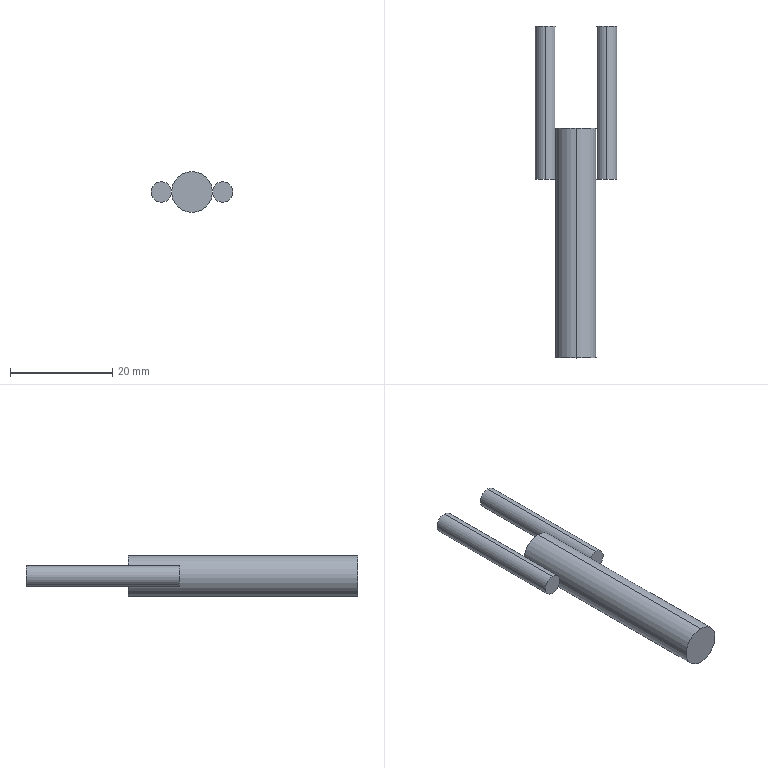Part | 3 solids | 12 faces | box 16 x 65 x 8 mm | volume 3016 mm3 | cylinder 6 | plane 6 | commonest cylinder face diameters 4 x4 8 x2
STEP:
#1=CARTESIAN_POINT('',(0.,45.,4.));
#2=VERTEX_POINT('',#1);
#3=CARTESIAN_POINT('',(0.,45.,-4.));
#4=VERTEX_POINT('',#3);
#5=CARTESIAN_POINT('',(0.,45.,0.));
#6=DIRECTION('',(0.,1.,0.));
#7=DIRECTION('',(0.,0.,1.));
#8=AXIS2_PLACEMENT_3D('',#5,#6,#7);
#9=CIRCLE('',#8,4.);
#10=EDGE_CURVE('',#2,#4,#9,.T.);
#11=ORIENTED_EDGE('',*,*,#10,.F.);
#12=CARTESIAN_POINT('',(0.,0.,4.));
#13=VERTEX_POINT('',#12);
#14=CARTESIAN_POINT('',(0.,45.,4.));
#15=DIRECTION('',(0.,-1.,0.));
#16=VECTOR('',#15,1000.);
#17=LINE('',#14,#16);
#18=EDGE_CURVE('',#2,#13,#17,.T.);
#19=ORIENTED_EDGE('',*,*,#18,.T.);
#20=CARTESIAN_POINT('',(0.,0.,-4.));
#21=VERTEX_POINT('',#20);
#22=CARTESIAN_POINT('',(0.,0.,0.));
#23=DIRECTION('',(0.,1.,0.));
#24=DIRECTION('',(0.,0.,1.));
#25=AXIS2_PLACEMENT_3D('',#22,#23,#24);
#26=CIRCLE('',#25,4.);
#27=EDGE_CURVE('',#13,#21,#26,.T.);
#28=ORIENTED_EDGE('',*,*,#27,.T.);
#29=CARTESIAN_POINT('',(0.,45.,-4.));
#30=DIRECTION('',(0.,-1.,0.));
#31=VECTOR('',#30,1000.);
#32=LINE('',#29,#31);
#33=EDGE_CURVE('',#4,#21,#32,.T.);
#34=ORIENTED_EDGE('',*,*,#33,.F.);
#35=EDGE_LOOP('',(#11,#19,#28,#34));
#36=FACE_OUTER_BOUND('',#35,.T.);
#37=CARTESIAN_POINT('',(0.,45.,0.));
#38=DIRECTION('',(0.,-1.,0.));
#39=DIRECTION('',(0.,0.,-1.));
#40=AXIS2_PLACEMENT_3D('',#37,#38,#39);
#41=CYLINDRICAL_SURFACE('',#40,4.);
#42=ADVANCED_FACE('',(#36),#41,.T.);
#43=ORIENTED_EDGE('',*,*,#18,.F.);
#44=CARTESIAN_POINT('',(0.,45.,0.));
#45=DIRECTION('',(0.,1.,0.));
#46=DIRECTION('',(0.,0.,1.));
#47=AXIS2_PLACEMENT_3D('',#44,#45,#46);
#48=CIRCLE('',#47,4.);
#49=EDGE_CURVE('',#4,#2,#48,.T.);
#50=ORIENTED_EDGE('',*,*,#49,.F.);
#51=ORIENTED_EDGE('',*,*,#33,.T.);
#52=CARTESIAN_POINT('',(0.,0.,0.));
#53=DIRECTION('',(0.,1.,0.));
#54=DIRECTION('',(0.,0.,1.));
#55=AXIS2_PLACEMENT_3D('',#52,#53,#54);
#56=CIRCLE('',#55,4.);
#57=EDGE_CURVE('',#21,#13,#56,.T.);
#58=ORIENTED_EDGE('',*,*,#57,.T.);
#59=EDGE_LOOP('',(#43,#50,#51,#58));
#60=FACE_OUTER_BOUND('',#59,.T.);
#61=CARTESIAN_POINT('',(0.,45.,0.));
#62=DIRECTION('',(0.,-1.,0.));
#63=DIRECTION('',(0.,0.,-1.));
#64=AXIS2_PLACEMENT_3D('',#61,#62,#63);
#65=CYLINDRICAL_SURFACE('',#64,4.);
#66=ADVANCED_FACE('',(#60),#65,.T.);
#67=ORIENTED_EDGE('',*,*,#49,.T.);
#68=ORIENTED_EDGE('',*,*,#10,.T.);
#69=EDGE_LOOP('',(#67,#68));
#70=FACE_OUTER_BOUND('',#69,.T.);
#71=CARTESIAN_POINT('',(0.,45.,0.));
#72=DIRECTION('',(0.,1.,0.));
#73=DIRECTION('',(0.,0.,1.));
#74=AXIS2_PLACEMENT_3D('',#71,#72,#73);
#75=PLANE('',#74);
#76=ADVANCED_FACE('',(#70),#75,.T.);
#77=ORIENTED_EDGE('',*,*,#57,.F.);
#78=ORIENTED_EDGE('',*,*,#27,.F.);
#79=EDGE_LOOP('',(#77,#78));
#80=FACE_OUTER_BOUND('',#79,.T.);
#81=CARTESIAN_POINT('',(0.,0.,0.));
#82=DIRECTION('',(0.,1.,0.));
#83=DIRECTION('',(0.,0.,1.));
#84=AXIS2_PLACEMENT_3D('',#81,#82,#83);
#85=PLANE('',#84);
#86=ADVANCED_FACE('',(#80),#85,.F.);
#87=CLOSED_SHELL('',(#42,#66,#76,#86));
#88=MANIFOLD_SOLID_BREP('',#87);
#89=CARTESIAN_POINT('',(-6.,65.,2.));
#90=VERTEX_POINT('',#89);
#91=CARTESIAN_POINT('',(-6.,65.,-2.));
#92=VERTEX_POINT('',#91);
#93=CARTESIAN_POINT('',(-6.,65.,0.));
#94=DIRECTION('',(0.,1.,0.));
#95=DIRECTION('',(0.,0.,1.));
#96=AXIS2_PLACEMENT_3D('',#93,#94,#95);
#97=CIRCLE('',#96,2.);
#98=EDGE_CURVE('',#90,#92,#97,.T.);
#99=ORIENTED_EDGE('',*,*,#98,.F.);
#100=CARTESIAN_POINT('',(-6.,35.,2.));
#101=VERTEX_POINT('',#100);
#102=CARTESIAN_POINT('',(-6.,65.,2.));
#103=DIRECTION('',(0.,-1.,0.));
#104=VECTOR('',#103,1000.);
#105=LINE('',#102,#104);
#106=EDGE_CURVE('',#90,#101,#105,.T.);
#107=ORIENTED_EDGE('',*,*,#106,.T.);
#108=CARTESIAN_POINT('',(-6.,35.,-2.));
#109=VERTEX_POINT('',#108);
#110=CARTESIAN_POINT('',(-6.,35.,0.));
#111=DIRECTION('',(0.,1.,0.));
#112=DIRECTION('',(0.,0.,1.));
#113=AXIS2_PLACEMENT_3D('',#110,#111,#112);
#114=CIRCLE('',#113,2.);
#115=EDGE_CURVE('',#101,#109,#114,.T.);
#116=ORIENTED_EDGE('',*,*,#115,.T.);
#117=CARTESIAN_POINT('',(-6.,65.,-2.));
#118=DIRECTION('',(0.,-1.,0.));
#119=VECTOR('',#118,1000.);
#120=LINE('',#117,#119);
#121=EDGE_CURVE('',#92,#109,#120,.T.);
#122=ORIENTED_EDGE('',*,*,#121,.F.);
#123=EDGE_LOOP('',(#99,#107,#116,#122));
#124=FACE_OUTER_BOUND('',#123,.T.);
#125=CARTESIAN_POINT('',(-6.,65.,0.));
#126=DIRECTION('',(0.,-1.,0.));
#127=DIRECTION('',(0.,0.,-1.));
#128=AXIS2_PLACEMENT_3D('',#125,#126,#127);
#129=CYLINDRICAL_SURFACE('',#128,2.);
#130=ADVANCED_FACE('',(#124),#129,.T.);
#131=ORIENTED_EDGE('',*,*,#106,.F.);
#132=CARTESIAN_POINT('',(-6.,65.,0.));
#133=DIRECTION('',(0.,1.,0.));
#134=DIRECTION('',(0.,0.,1.));
#135=AXIS2_PLACEMENT_3D('',#132,#133,#134);
#136=CIRCLE('',#135,2.);
#137=EDGE_CURVE('',#92,#90,#136,.T.);
#138=ORIENTED_EDGE('',*,*,#137,.F.);
#139=ORIENTED_EDGE('',*,*,#121,.T.);
#140=CARTESIAN_POINT('',(-6.,35.,0.));
#141=DIRECTION('',(0.,1.,0.));
#142=DIRECTION('',(0.,0.,1.));
#143=AXIS2_PLACEMENT_3D('',#140,#141,#142);
#144=CIRCLE('',#143,2.);
#145=EDGE_CURVE('',#109,#101,#144,.T.);
#146=ORIENTED_EDGE('',*,*,#145,.T.);
#147=EDGE_LOOP('',(#131,#138,#139,#146));
#148=FACE_OUTER_BOUND('',#147,.T.);
#149=CARTESIAN_POINT('',(-6.,65.,0.));
#150=DIRECTION('',(0.,-1.,0.));
#151=DIRECTION('',(0.,0.,-1.));
#152=AXIS2_PLACEMENT_3D('',#149,#150,#151);
#153=CYLINDRICAL_SURFACE('',#152,2.);
#154=ADVANCED_FACE('',(#148),#153,.T.);
#155=ORIENTED_EDGE('',*,*,#137,.T.);
#156=ORIENTED_EDGE('',*,*,#98,.T.);
#157=EDGE_LOOP('',(#155,#156));
#158=FACE_OUTER_BOUND('',#157,.T.);
#159=CARTESIAN_POINT('',(-6.,65.,0.));
#160=DIRECTION('',(0.,1.,0.));
#161=DIRECTION('',(0.,0.,1.));
#162=AXIS2_PLACEMENT_3D('',#159,#160,#161);
#163=PLANE('',#162);
#164=ADVANCED_FACE('',(#158),#163,.T.);
#165=ORIENTED_EDGE('',*,*,#145,.F.);
#166=ORIENTED_EDGE('',*,*,#115,.F.);
#167=EDGE_LOOP('',(#165,#166));
#168=FACE_OUTER_BOUND('',#167,.T.);
#169=CARTESIAN_POINT('',(-6.,35.,0.));
#170=DIRECTION('',(0.,1.,0.));
#171=DIRECTION('',(0.,0.,1.));
#172=AXIS2_PLACEMENT_3D('',#169,#170,#171);
#173=PLANE('',#172);
#174=ADVANCED_FACE('',(#168),#173,.F.);
#175=CLOSED_SHELL('',(#130,#154,#164,#174));
#176=MANIFOLD_SOLID_BREP('',#175);
#177=CARTESIAN_POINT('',(6.,65.,2.));
#178=VERTEX_POINT('',#177);
#179=CARTESIAN_POINT('',(6.,65.,-2.));
#180=VERTEX_POINT('',#179);
#181=CARTESIAN_POINT('',(6.,65.,0.));
#182=DIRECTION('',(0.,1.,0.));
#183=DIRECTION('',(0.,0.,-1.));
#184=AXIS2_PLACEMENT_3D('',#181,#182,#183);
#185=CIRCLE('',#184,2.);
#186=EDGE_CURVE('',#178,#180,#185,.T.);
#187=ORIENTED_EDGE('',*,*,#186,.F.);
#188=CARTESIAN_POINT('',(6.,35.,2.));
#189=VERTEX_POINT('',#188);
#190=CARTESIAN_POINT('',(6.,65.,2.));
#191=DIRECTION('',(0.,-1.,0.));
#192=VECTOR('',#191,1000.);
#193=LINE('',#190,#192);
#194=EDGE_CURVE('',#178,#189,#193,.T.);
#195=ORIENTED_EDGE('',*,*,#194,.T.);
#196=CARTESIAN_POINT('',(6.,35.,-2.));
#197=VERTEX_POINT('',#196);
#198=CARTESIAN_POINT('',(6.,35.,0.));
#199=DIRECTION('',(0.,1.,0.));
#200=DIRECTION('',(0.,0.,-1.));
#201=AXIS2_PLACEMENT_3D('',#198,#199,#200);
#202=CIRCLE('',#201,2.);
#203=EDGE_CURVE('',#189,#197,#202,.T.);
#204=ORIENTED_EDGE('',*,*,#203,.T.);
#205=CARTESIAN_POINT('',(6.,65.,-2.));
#206=DIRECTION('',(0.,-1.,0.));
#207=VECTOR('',#206,1000.);
#208=LINE('',#205,#207);
#209=EDGE_CURVE('',#180,#197,#208,.T.);
#210=ORIENTED_EDGE('',*,*,#209,.F.);
#211=EDGE_LOOP('',(#187,#195,#204,#210));
#212=FACE_OUTER_BOUND('',#211,.T.);
#213=CARTESIAN_POINT('',(6.,65.,0.));
#214=DIRECTION('',(0.,-1.,0.));
#215=DIRECTION('',(0.,0.,-1.));
#216=AXIS2_PLACEMENT_3D('',#213,#214,#215);
#217=CYLINDRICAL_SURFACE('',#216,2.);
#218=ADVANCED_FACE('',(#212),#217,.T.);
#219=ORIENTED_EDGE('',*,*,#194,.F.);
#220=CARTESIAN_POINT('',(6.,65.,0.));
#221=DIRECTION('',(0.,1.,0.));
#222=DIRECTION('',(0.,0.,-1.));
#223=AXIS2_PLACEMENT_3D('',#220,#221,#222);
#224=CIRCLE('',#223,2.);
#225=EDGE_CURVE('',#180,#178,#224,.T.);
#226=ORIENTED_EDGE('',*,*,#225,.F.);
#227=ORIENTED_EDGE('',*,*,#209,.T.);
#228=CARTESIAN_POINT('',(6.,35.,0.));
#229=DIRECTION('',(0.,1.,0.));
#230=DIRECTION('',(0.,0.,-1.));
#231=AXIS2_PLACEMENT_3D('',#228,#229,#230);
#232=CIRCLE('',#231,2.);
#233=EDGE_CURVE('',#197,#189,#232,.T.);
#234=ORIENTED_EDGE('',*,*,#233,.T.);
#235=EDGE_LOOP('',(#219,#226,#227,#234));
#236=FACE_OUTER_BOUND('',#235,.T.);
#237=CARTESIAN_POINT('',(6.,65.,0.));
#238=DIRECTION('',(0.,-1.,0.));
#239=DIRECTION('',(0.,0.,-1.));
#240=AXIS2_PLACEMENT_3D('',#237,#238,#239);
#241=CYLINDRICAL_SURFACE('',#240,2.);
#242=ADVANCED_FACE('',(#236),#241,.T.);
#243=ORIENTED_EDGE('',*,*,#225,.T.);
#244=ORIENTED_EDGE('',*,*,#186,.T.);
#245=EDGE_LOOP('',(#243,#244));
#246=FACE_OUTER_BOUND('',#245,.T.);
#247=CARTESIAN_POINT('',(6.,65.,0.));
#248=DIRECTION('',(0.,-1.,0.));
#249=DIRECTION('',(0.,0.,-1.));
#250=AXIS2_PLACEMENT_3D('',#247,#248,#249);
#251=PLANE('',#250);
#252=ADVANCED_FACE('',(#246),#251,.F.);
#253=ORIENTED_EDGE('',*,*,#233,.F.);
#254=ORIENTED_EDGE('',*,*,#203,.F.);
#255=EDGE_LOOP('',(#253,#254));
#256=FACE_OUTER_BOUND('',#255,.T.);
#257=CARTESIAN_POINT('',(6.,35.,0.));
#258=DIRECTION('',(0.,-1.,0.));
#259=DIRECTION('',(0.,0.,-1.));
#260=AXIS2_PLACEMENT_3D('',#257,#258,#259);
#261=PLANE('',#260);
#262=ADVANCED_FACE('',(#256),#261,.T.);
#263=CLOSED_SHELL('',(#218,#242,#252,#262));
#264=MANIFOLD_SOLID_BREP('',#263);
#265=CARTESIAN_POINT('',(0.,0.,0.));
#266=DIRECTION('',(0.,0.,1.));
#267=DIRECTION('',(1.,0.,0.));
#268=AXIS2_PLACEMENT_3D('',#265,#266,#267);
#269=(LENGTH_UNIT()NAMED_UNIT(*)SI_UNIT(.MILLI.,.METRE.));
#270=UNCERTAINTY_MEASURE_WITH_UNIT(LENGTH_MEASURE(0.00001),#269,'','');
#271=(NAMED_UNIT(*)PLANE_ANGLE_UNIT()SI_UNIT($,.RADIAN.));
#272=(NAMED_UNIT(*)SI_UNIT($,.STERADIAN.)SOLID_ANGLE_UNIT());
#273=(GEOMETRIC_REPRESENTATION_CONTEXT(3)GLOBAL_UNCERTAINTY_ASSIGNED_CONTEXT((#270))GLOBAL_UNIT_ASSIGNED_CONTEXT((#269,#271,#272))REPRESENTATION_CONTEXT('',''));
#274=ADVANCED_BREP_SHAPE_REPRESENTATION('',(#88,#176,#264,#268),#273);